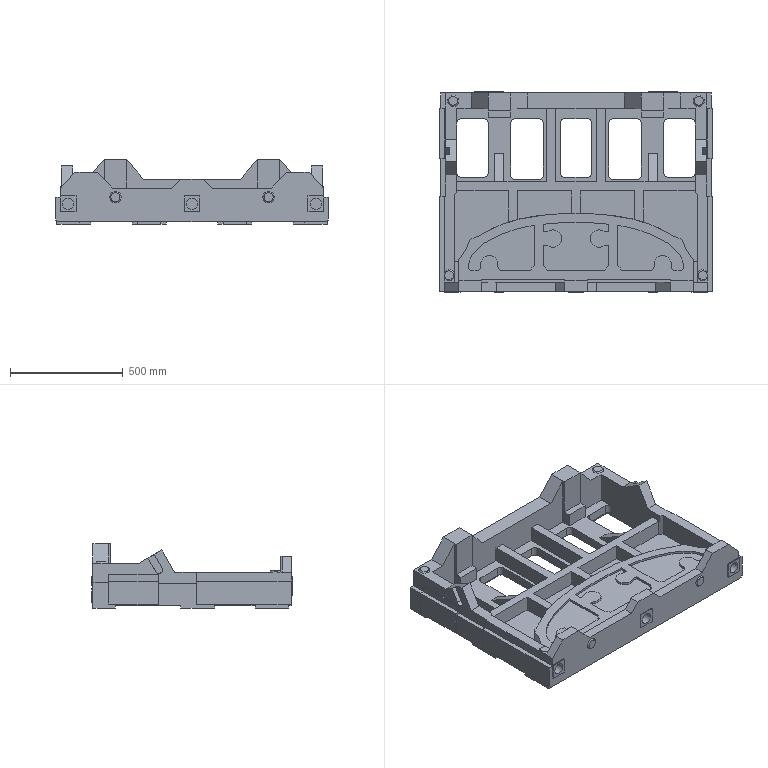Part | NX | features solid 2 | 1 solid | 430 faces | box 1210 x 890 x 285 mm | volume 82458161 mm3 | plane 352 | cylinder 56 | spline 14 | cone 8 | commonest cylinder face diameters 40 x30 77 x8 50 x7 105 x6 32 x2 50.2 x2